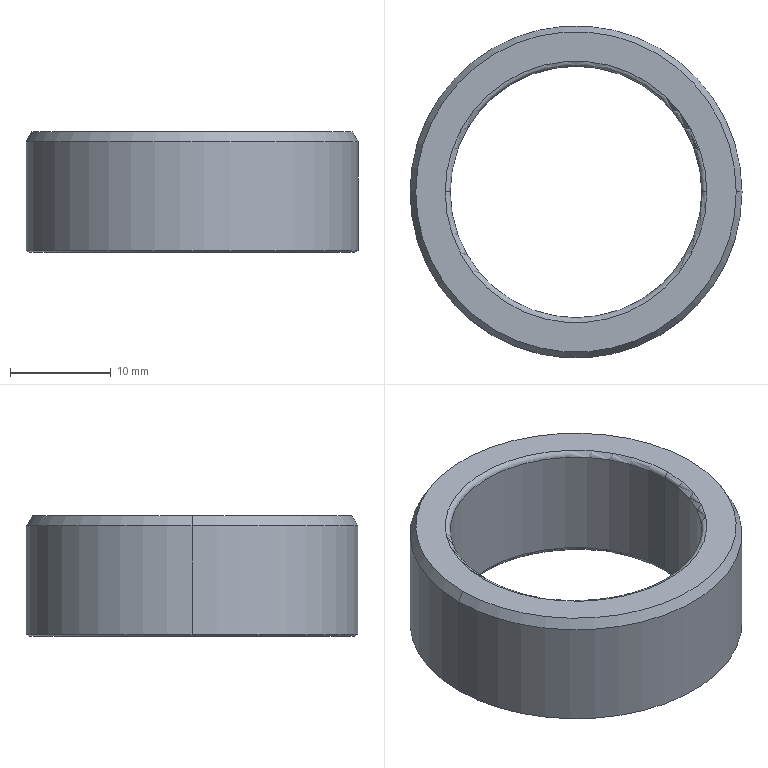Part | STEP file | Graphite bronze bushing JDB253312 | 1 solid | 14 faces | box 33 x 33 x 12 mm | volume 4332 mm3 | torus 4 | cone 4 | cylinder 4 | plane 2 | commonest cylinder face diameters 25 x2 33 x2
STEP:
#1=CARTESIAN_POINT('',(0.,0.,0.));
#2=DIRECTION('',(0.,0.,1.));
#3=DIRECTION('',(1.,0.,0.));
#4=AXIS2_PLACEMENT_3D('',#1,#2,#3);
#5=CARTESIAN_POINT('',(-12.5,0.,-5.5));
#6=VERTEX_POINT('',#5);
#7=CARTESIAN_POINT('',(12.5,0.,-5.5));
#8=VERTEX_POINT('',#7);
#9=CARTESIAN_POINT('',(0.,0.,-5.5));
#10=DIRECTION('',(0.,0.,-1.));
#11=DIRECTION('',(1.,0.,0.));
#12=AXIS2_PLACEMENT_3D('',#9,#10,#11);
#13=CIRCLE('',#12,12.5);
#14=CARTESIAN_POINT('',(0.,0.,-5.5));
#15=DIRECTION('',(0.,0.,1.));
#16=DIRECTION('',(1.,0.,0.));
#17=AXIS2_PLACEMENT_3D('',#14,#15,#16);
#18=TOROIDAL_SURFACE('',#17,13.,0.5);
#19=CARTESIAN_POINT('',(6.283,3.142));
#20=DIRECTION('',(-1.,0.));
#21=VECTOR('',#20,1.);
#22=LINE('',#19,#21);
#23=(GEOMETRIC_REPRESENTATION_CONTEXT(2)PARAMETRIC_REPRESENTATION_CONTEXT()REPRESENTATION_CONTEXT('',''));
#24=DEFINITIONAL_REPRESENTATION('',(#22),#23);
#25=PCURVE('',#18,#24);
#26=CARTESIAN_POINT('',(0.,0.,6.));
#27=DIRECTION('',(0.,0.,-1.));
#28=DIRECTION('',(-1.,0.,0.));
#29=AXIS2_PLACEMENT_3D('',#26,#27,#28);
#30=CYLINDRICAL_SURFACE('',#29,12.5);
#31=CARTESIAN_POINT('',(-3.142,11.5));
#32=DIRECTION('',(1.,0.));
#33=VECTOR('',#32,1.);
#34=LINE('',#31,#33);
#35=(GEOMETRIC_REPRESENTATION_CONTEXT(2)PARAMETRIC_REPRESENTATION_CONTEXT()REPRESENTATION_CONTEXT('',''));
#36=DEFINITIONAL_REPRESENTATION('',(#34),#35);
#37=PCURVE('',#30,#36);
#38=SURFACE_CURVE('',#13,(#25,#37),.PCURVE_S1.);
#39=EDGE_CURVE('',#6,#8,#38,.T.);
#40=ORIENTED_EDGE('',*,*,#39,.F.);
#41=CARTESIAN_POINT('',(-13.,0.,-6.));
#42=VERTEX_POINT('',#41);
#43=CARTESIAN_POINT('',(-13.,0.,-5.5));
#44=DIRECTION('',(0.,1.,0.));
#45=DIRECTION('',(-1.,0.,0.));
#46=AXIS2_PLACEMENT_3D('',#43,#44,#45);
#47=CIRCLE('',#46,0.5);
#48=CARTESIAN_POINT('',(3.142,0.));
#49=DIRECTION('',(0.,1.));
#50=VECTOR('',#49,1.);
#51=LINE('',#48,#50);
#52=(GEOMETRIC_REPRESENTATION_CONTEXT(2)PARAMETRIC_REPRESENTATION_CONTEXT()REPRESENTATION_CONTEXT('',''));
#53=DEFINITIONAL_REPRESENTATION('',(#51),#52);
#54=PCURVE('',#18,#53);
#55=CARTESIAN_POINT('',(0.,0.,-5.5));
#56=DIRECTION('',(0.,0.,1.));
#57=DIRECTION('',(1.,0.,0.));
#58=AXIS2_PLACEMENT_3D('',#55,#56,#57);
#59=TOROIDAL_SURFACE('',#58,13.,0.5);
#60=CARTESIAN_POINT('',(3.142,0.));
#61=DIRECTION('',(0.,1.));
#62=VECTOR('',#61,1.);
#63=LINE('',#60,#62);
#64=(GEOMETRIC_REPRESENTATION_CONTEXT(2)PARAMETRIC_REPRESENTATION_CONTEXT()REPRESENTATION_CONTEXT('',''));
#65=DEFINITIONAL_REPRESENTATION('',(#63),#64);
#66=PCURVE('',#59,#65);
#67=SURFACE_CURVE('',#47,(#54,#66),.PCURVE_S1.);
#68=EDGE_CURVE('',#6,#42,#67,.T.);
#69=ORIENTED_EDGE('',*,*,#68,.T.);
#70=CARTESIAN_POINT('',(13.,0.,-6.));
#71=VERTEX_POINT('',#70);
#72=CARTESIAN_POINT('',(0.,0.,-6.));
#73=DIRECTION('',(0.,0.,1.));
#74=DIRECTION('',(1.,0.,0.));
#75=AXIS2_PLACEMENT_3D('',#72,#73,#74);
#76=CIRCLE('',#75,13.);
#77=CARTESIAN_POINT('',(0.,4.712));
#78=DIRECTION('',(1.,0.));
#79=VECTOR('',#78,1.);
#80=LINE('',#77,#79);
#81=(GEOMETRIC_REPRESENTATION_CONTEXT(2)PARAMETRIC_REPRESENTATION_CONTEXT()REPRESENTATION_CONTEXT('',''));
#82=DEFINITIONAL_REPRESENTATION('',(#80),#81);
#83=PCURVE('',#18,#82);
#84=CARTESIAN_POINT('',(0.,0.,-6.));
#85=DIRECTION('',(0.,0.,1.));
#86=DIRECTION('',(1.,0.,0.));
#87=AXIS2_PLACEMENT_3D('',#84,#85,#86);
#88=PLANE('',#87);
#89=CARTESIAN_POINT('',(0.,0.));
#90=DIRECTION('',(1.,0.));
#91=AXIS2_PLACEMENT_2D('',#89,#90);
#92=CIRCLE('',#91,13.);
#93=(GEOMETRIC_REPRESENTATION_CONTEXT(2)PARAMETRIC_REPRESENTATION_CONTEXT()REPRESENTATION_CONTEXT('',''));
#94=DEFINITIONAL_REPRESENTATION('',(#92),#93);
#95=PCURVE('',#88,#94);
#96=SURFACE_CURVE('',#76,(#83,#95),.PCURVE_S1.);
#97=EDGE_CURVE('',#71,#42,#96,.T.);
#98=ORIENTED_EDGE('',*,*,#97,.F.);
#99=CARTESIAN_POINT('',(13.,0.,-5.5));
#100=DIRECTION('',(0.,-1.,0.));
#101=DIRECTION('',(0.,0.,-1.));
#102=AXIS2_PLACEMENT_3D('',#99,#100,#101);
#103=CIRCLE('',#102,0.5);
#104=CARTESIAN_POINT('',(0.,-1.571));
#105=DIRECTION('',(0.,1.));
#106=VECTOR('',#105,1.);
#107=LINE('',#104,#106);
#108=(GEOMETRIC_REPRESENTATION_CONTEXT(2)PARAMETRIC_REPRESENTATION_CONTEXT()REPRESENTATION_CONTEXT('',''));
#109=DEFINITIONAL_REPRESENTATION('',(#107),#108);
#110=PCURVE('',#18,#109);
#111=CARTESIAN_POINT('',(6.283,-1.571));
#112=DIRECTION('',(0.,1.));
#113=VECTOR('',#112,1.);
#114=LINE('',#111,#113);
#115=(GEOMETRIC_REPRESENTATION_CONTEXT(2)PARAMETRIC_REPRESENTATION_CONTEXT()REPRESENTATION_CONTEXT('',''));
#116=DEFINITIONAL_REPRESENTATION('',(#114),#115);
#117=PCURVE('',#59,#116);
#118=SURFACE_CURVE('',#103,(#110,#117),.PCURVE_S1.);
#119=EDGE_CURVE('',#8,#71,#118,.T.);
#120=ORIENTED_EDGE('',*,*,#119,.F.);
#121=EDGE_LOOP('',(#40,#69,#98,#120));
#122=FACE_BOUND('',#121,.T.);
#123=ADVANCED_FACE('',(#122),#18,.T.);
#124=CARTESIAN_POINT('',(-13.,0.,6.));
#125=VERTEX_POINT('',#124);
#126=CARTESIAN_POINT('',(13.,0.,6.));
#127=VERTEX_POINT('',#126);
#128=CARTESIAN_POINT('',(0.,0.,6.));
#129=DIRECTION('',(0.,0.,-1.));
#130=DIRECTION('',(1.,0.,0.));
#131=AXIS2_PLACEMENT_3D('',#128,#129,#130);
#132=CIRCLE('',#131,13.);
#133=CARTESIAN_POINT('',(0.,0.,5.5));
#134=DIRECTION('',(0.,0.,1.));
#135=DIRECTION('',(1.,0.,0.));
#136=AXIS2_PLACEMENT_3D('',#133,#134,#135);
#137=TOROIDAL_SURFACE('',#136,13.,0.5);
#138=CARTESIAN_POINT('',(6.283,1.571));
#139=DIRECTION('',(-1.,0.));
#140=VECTOR('',#139,1.);
#141=LINE('',#138,#140);
#142=(GEOMETRIC_REPRESENTATION_CONTEXT(2)PARAMETRIC_REPRESENTATION_CONTEXT()REPRESENTATION_CONTEXT('',''));
#143=DEFINITIONAL_REPRESENTATION('',(#141),#142);
#144=PCURVE('',#137,#143);
#145=CARTESIAN_POINT('',(0.,0.,6.));
#146=DIRECTION('',(0.,0.,1.));
#147=DIRECTION('',(1.,0.,0.));
#148=AXIS2_PLACEMENT_3D('',#145,#146,#147);
#149=PLANE('',#148);
#150=CARTESIAN_POINT('',(13.,0.));
#151=CARTESIAN_POINT('',(13.,-22.517));
#152=CARTESIAN_POINT('',(-6.5,-11.258));
#153=CARTESIAN_POINT('',(-26.,0.));
#154=CARTESIAN_POINT('',(-6.5,11.258));
#155=CARTESIAN_POINT('',(13.,22.517));
#156=CARTESIAN_POINT('',(13.,0.));
#157=(BOUNDED_CURVE()B_SPLINE_CURVE(2,(#150,#151,#152,#153,#154,#155,#156),.UNSPECIFIED.,.T.,.F.)B_SPLINE_CURVE_WITH_KNOTS((1,2,2,2,2,1),(-2.094,0.,2.094,4.189,6.283,8.378),.UNSPECIFIED.)CURVE()GEOMETRIC_REPRESENTATION_ITEM()RATIONAL_B_SPLINE_CURVE((1.,0.5,1.,0.5,1.,0.5,1.))REPRESENTATION_ITEM(''));
#158=(GEOMETRIC_REPRESENTATION_CONTEXT(2)PARAMETRIC_REPRESENTATION_CONTEXT()REPRESENTATION_CONTEXT('',''));
#159=DEFINITIONAL_REPRESENTATION('',(#157),#158);
#160=PCURVE('',#149,#159);
#161=SURFACE_CURVE('',#132,(#144,#160),.PCURVE_S1.);
#162=EDGE_CURVE('',#125,#127,#161,.T.);
#163=ORIENTED_EDGE('',*,*,#162,.F.);
#164=CARTESIAN_POINT('',(-12.5,0.,5.5));
#165=VERTEX_POINT('',#164);
#166=CARTESIAN_POINT('',(-13.,0.,5.5));
#167=DIRECTION('',(0.,1.,0.));
#168=DIRECTION('',(-1.,0.,0.));
#169=AXIS2_PLACEMENT_3D('',#166,#167,#168);
#170=CIRCLE('',#169,0.5);
#171=CARTESIAN_POINT('',(3.142,0.));
#172=DIRECTION('',(0.,1.));
#173=VECTOR('',#172,1.);
#174=LINE('',#171,#173);
#175=(GEOMETRIC_REPRESENTATION_CONTEXT(2)PARAMETRIC_REPRESENTATION_CONTEXT()REPRESENTATION_CONTEXT('',''));
#176=DEFINITIONAL_REPRESENTATION('',(#174),#175);
#177=PCURVE('',#137,#176);
#178=CARTESIAN_POINT('',(0.,0.,5.5));
#179=DIRECTION('',(0.,0.,1.));
#180=DIRECTION('',(1.,0.,0.));
#181=AXIS2_PLACEMENT_3D('',#178,#179,#180);
#182=TOROIDAL_SURFACE('',#181,13.,0.5);
#183=CARTESIAN_POINT('',(3.142,0.));
#184=DIRECTION('',(0.,1.));
#185=VECTOR('',#184,1.);
#186=LINE('',#183,#185);
#187=(GEOMETRIC_REPRESENTATION_CONTEXT(2)PARAMETRIC_REPRESENTATION_CONTEXT()REPRESENTATION_CONTEXT('',''));
#188=DEFINITIONAL_REPRESENTATION('',(#186),#187);
#189=PCURVE('',#182,#188);
#190=SURFACE_CURVE('',#170,(#177,#189),.PCURVE_S1.);
#191=EDGE_CURVE('',#125,#165,#190,.T.);
#192=ORIENTED_EDGE('',*,*,#191,.T.);
#193=CARTESIAN_POINT('',(12.5,0.,5.5));
#194=VERTEX_POINT('',#193);
#195=CARTESIAN_POINT('',(0.,0.,5.5));
#196=DIRECTION('',(0.,0.,1.));
#197=DIRECTION('',(1.,0.,0.));
#198=AXIS2_PLACEMENT_3D('',#195,#196,#197);
#199=CIRCLE('',#198,12.5);
#200=CARTESIAN_POINT('',(0.,3.142));
#201=DIRECTION('',(1.,0.));
#202=VECTOR('',#201,1.);
#203=LINE('',#200,#202);
#204=(GEOMETRIC_REPRESENTATION_CONTEXT(2)PARAMETRIC_REPRESENTATION_CONTEXT()REPRESENTATION_CONTEXT('',''));
#205=DEFINITIONAL_REPRESENTATION('',(#203),#204);
#206=PCURVE('',#137,#205);
#207=CARTESIAN_POINT('',(3.142,0.5));
#208=DIRECTION('',(-1.,0.));
#209=VECTOR('',#208,1.);
#210=LINE('',#207,#209);
#211=(GEOMETRIC_REPRESENTATION_CONTEXT(2)PARAMETRIC_REPRESENTATION_CONTEXT()REPRESENTATION_CONTEXT('',''));
#212=DEFINITIONAL_REPRESENTATION('',(#210),#211);
#213=PCURVE('',#30,#212);
#214=SURFACE_CURVE('',#199,(#206,#213),.PCURVE_S1.);
#215=EDGE_CURVE('',#194,#165,#214,.T.);
#216=ORIENTED_EDGE('',*,*,#215,.F.);
#217=CARTESIAN_POINT('',(13.,0.,5.5));
#218=DIRECTION('',(0.,-1.,0.));
#219=DIRECTION('',(0.,0.,-1.));
#220=AXIS2_PLACEMENT_3D('',#217,#218,#219);
#221=CIRCLE('',#220,0.5);
#222=CARTESIAN_POINT('',(0.,-1.571));
#223=DIRECTION('',(0.,1.));
#224=VECTOR('',#223,1.);
#225=LINE('',#222,#224);
#226=(GEOMETRIC_REPRESENTATION_CONTEXT(2)PARAMETRIC_REPRESENTATION_CONTEXT()REPRESENTATION_CONTEXT('',''));
#227=DEFINITIONAL_REPRESENTATION('',(#225),#226);
#228=PCURVE('',#137,#227);
#229=CARTESIAN_POINT('',(6.283,-1.571));
#230=DIRECTION('',(0.,1.));
#231=VECTOR('',#230,1.);
#232=LINE('',#229,#231);
#233=(GEOMETRIC_REPRESENTATION_CONTEXT(2)PARAMETRIC_REPRESENTATION_CONTEXT()REPRESENTATION_CONTEXT('',''));
#234=DEFINITIONAL_REPRESENTATION('',(#232),#233);
#235=PCURVE('',#182,#234);
#236=SURFACE_CURVE('',#221,(#228,#235),.PCURVE_S1.);
#237=EDGE_CURVE('',#127,#194,#236,.T.);
#238=ORIENTED_EDGE('',*,*,#237,.F.);
#239=EDGE_LOOP('',(#163,#192,#216,#238));
#240=FACE_BOUND('',#239,.T.);
#241=ADVANCED_FACE('',(#240),#137,.T.);
#242=CARTESIAN_POINT('',(-16.2,0.,-6.));
#243=VERTEX_POINT('',#242);
#244=CARTESIAN_POINT('',(16.2,0.,-6.));
#245=VERTEX_POINT('',#244);
#246=CARTESIAN_POINT('',(0.,0.,-6.));
#247=DIRECTION('',(0.,0.,-1.));
#248=DIRECTION('',(1.,0.,0.));
#249=AXIS2_PLACEMENT_3D('',#246,#247,#248);
#250=CIRCLE('',#249,16.2);
#251=CARTESIAN_POINT('',(0.,0.,-5.827));
#252=DIRECTION('',(0.,0.,1.));
#253=DIRECTION('',(1.,0.,0.));
#254=AXIS2_PLACEMENT_3D('',#251,#252,#253);
#255=CONICAL_SURFACE('',#254,16.5,1.047);
#256=CARTESIAN_POINT('',(6.283,-0.1732));
#257=DIRECTION('',(-1.,0.));
#258=VECTOR('',#257,1.);
#259=LINE('',#256,#258);
#260=(GEOMETRIC_REPRESENTATION_CONTEXT(2)PARAMETRIC_REPRESENTATION_CONTEXT()REPRESENTATION_CONTEXT('',''));
#261=DEFINITIONAL_REPRESENTATION('',(#259),#260);
#262=PCURVE('',#255,#261);
#263=CARTESIAN_POINT('',(16.2,0.));
#264=CARTESIAN_POINT('',(16.2,-28.059));
#265=CARTESIAN_POINT('',(-8.1,-14.03));
#266=CARTESIAN_POINT('',(-32.4,0.));
#267=CARTESIAN_POINT('',(-8.1,14.03));
#268=CARTESIAN_POINT('',(16.2,28.059));
#269=CARTESIAN_POINT('',(16.2,0.));
#270=(BOUNDED_CURVE()B_SPLINE_CURVE(2,(#263,#264,#265,#266,#267,#268,#269),.UNSPECIFIED.,.T.,.F.)B_SPLINE_CURVE_WITH_KNOTS((1,2,2,2,2,1),(-2.094,0.,2.094,4.189,6.283,8.378),.UNSPECIFIED.)CURVE()GEOMETRIC_REPRESENTATION_ITEM()RATIONAL_B_SPLINE_CURVE((1.,0.5,1.,0.5,1.,0.5,1.))REPRESENTATION_ITEM(''));
#271=(GEOMETRIC_REPRESENTATION_CONTEXT(2)PARAMETRIC_REPRESENTATION_CONTEXT()REPRESENTATION_CONTEXT('',''));
#272=DEFINITIONAL_REPRESENTATION('',(#270),#271);
#273=PCURVE('',#88,#272);
#274=SURFACE_CURVE('',#250,(#262,#273),.PCURVE_S1.);
#275=EDGE_CURVE('',#243,#245,#274,.T.);
#276=ORIENTED_EDGE('',*,*,#275,.F.);
#277=CARTESIAN_POINT('',(-16.5,0.,-5.827));
#278=VERTEX_POINT('',#277);
#279=CARTESIAN_POINT('',(-16.5,0.,-5.827));
#280=DIRECTION('',(-0.866,0.,0.5));
#281=VECTOR('',#280,1.);
#282=LINE('',#279,#281);
#283=CARTESIAN_POINT('',(3.142,0.));
#284=DIRECTION('',(0.,1.));
#285=VECTOR('',#284,1.);
#286=LINE('',#283,#285);
#287=(GEOMETRIC_REPRESENTATION_CONTEXT(2)PARAMETRIC_REPRESENTATION_CONTEXT()REPRESENTATION_CONTEXT('',''));
#288=DEFINITIONAL_REPRESENTATION('',(#286),#287);
#289=PCURVE('',#255,#288);
#290=CARTESIAN_POINT('',(0.,0.,-5.827));
#291=DIRECTION('',(0.,0.,1.));
#292=DIRECTION('',(1.,0.,0.));
#293=AXIS2_PLACEMENT_3D('',#290,#291,#292);
#294=CONICAL_SURFACE('',#293,16.5,1.047);
#295=CARTESIAN_POINT('',(3.142,0.));
#296=DIRECTION('',(0.,1.));
#297=VECTOR('',#296,1.);
#298=LINE('',#295,#297);
#299=(GEOMETRIC_REPRESENTATION_CONTEXT(2)PARAMETRIC_REPRESENTATION_CONTEXT()REPRESENTATION_CONTEXT('',''));
#300=DEFINITIONAL_REPRESENTATION('',(#298),#299);
#301=PCURVE('',#294,#300);
#302=SURFACE_CURVE('',#282,(#289,#301),.PCURVE_S1.);
#303=EDGE_CURVE('',#243,#278,#302,.T.);
#304=ORIENTED_EDGE('',*,*,#303,.T.);
#305=CARTESIAN_POINT('',(16.5,0.,-5.827));
#306=VERTEX_POINT('',#305);
#307=CARTESIAN_POINT('',(0.,0.,-5.827));
#308=DIRECTION('',(0.,0.,1.));
#309=DIRECTION('',(1.,0.,0.));
#310=AXIS2_PLACEMENT_3D('',#307,#308,#309);
#311=CIRCLE('',#310,16.5);
#312=CARTESIAN_POINT('',(0.,0.));
#313=DIRECTION('',(1.,0.));
#314=VECTOR('',#313,1.);
#315=LINE('',#312,#314);
#316=(GEOMETRIC_REPRESENTATION_CONTEXT(2)PARAMETRIC_REPRESENTATION_CONTEXT()REPRESENTATION_CONTEXT('',''));
#317=DEFINITIONAL_REPRESENTATION('',(#315),#316);
#318=PCURVE('',#255,#317);
#319=CARTESIAN_POINT('',(0.,0.,6.));
#320=DIRECTION('',(0.,0.,-1.));
#321=DIRECTION('',(-1.,0.,0.));
#322=AXIS2_PLACEMENT_3D('',#319,#320,#321);
#323=CYLINDRICAL_SURFACE('',#322,16.5);
#324=CARTESIAN_POINT('',(3.142,11.827));
#325=DIRECTION('',(-1.,0.));
#326=VECTOR('',#325,1.);
#327=LINE('',#324,#326);
#328=(GEOMETRIC_REPRESENTATION_CONTEXT(2)PARAMETRIC_REPRESENTATION_CONTEXT()REPRESENTATION_CONTEXT('',''));
#329=DEFINITIONAL_REPRESENTATION('',(#327),#328);
#330=PCURVE('',#323,#329);
#331=SURFACE_CURVE('',#311,(#318,#330),.PCURVE_S1.);
#332=EDGE_CURVE('',#306,#278,#331,.T.);
#333=ORIENTED_EDGE('',*,*,#332,.F.);
#334=CARTESIAN_POINT('',(16.5,0.,-5.827));
#335=DIRECTION('',(0.866,0.,0.5));
#336=VECTOR('',#335,1.);
#337=LINE('',#334,#336);
#338=CARTESIAN_POINT('',(0.,0.));
#339=DIRECTION('',(0.,1.));
#340=VECTOR('',#339,1.);
#341=LINE('',#338,#340);
#342=(GEOMETRIC_REPRESENTATION_CONTEXT(2)PARAMETRIC_REPRESENTATION_CONTEXT()REPRESENTATION_CONTEXT('',''));
#343=DEFINITIONAL_REPRESENTATION('',(#341),#342);
#344=PCURVE('',#255,#343);
#345=CARTESIAN_POINT('',(6.283,0.));
#346=DIRECTION('',(0.,1.));
#347=VECTOR('',#346,1.);
#348=LINE('',#345,#347);
#349=(GEOMETRIC_REPRESENTATION_CONTEXT(2)PARAMETRIC_REPRESENTATION_CONTEXT()REPRESENTATION_CONTEXT('',''));
#350=DEFINITIONAL_REPRESENTATION('',(#348),#349);
#351=PCURVE('',#294,#350);
#352=SURFACE_CURVE('',#337,(#344,#351),.PCURVE_S1.);
#353=EDGE_CURVE('',#245,#306,#352,.T.);
#354=ORIENTED_EDGE('',*,*,#353,.F.);
#355=EDGE_LOOP('',(#276,#304,#333,#354));
#356=FACE_BOUND('',#355,.T.);
#357=ADVANCED_FACE('',(#356),#255,.T.);
#358=CARTESIAN_POINT('',(15.923,0.,6.));
#359=VERTEX_POINT('',#358);
#360=CARTESIAN_POINT('',(-15.923,0.,6.));
#361=VERTEX_POINT('',#360);
#362=CARTESIAN_POINT('',(0.,0.,6.));
#363=DIRECTION('',(0.,0.,1.));
#364=DIRECTION('',(1.,0.,0.));
#365=AXIS2_PLACEMENT_3D('',#362,#363,#364);
#366=CIRCLE('',#365,15.923);
#367=CARTESIAN_POINT('',(0.,0.,6.));
#368=DIRECTION('',(0.,0.,-1.));
#369=DIRECTION('',(-1.,0.,0.));
#370=AXIS2_PLACEMENT_3D('',#367,#368,#369);
#371=CONICAL_SURFACE('',#370,15.923,0.5236);
#372=CARTESIAN_POINT('',(3.142,0.));
#373=DIRECTION('',(-1.,0.));
#374=VECTOR('',#373,1.);
#375=LINE('',#372,#374);
#376=(GEOMETRIC_REPRESENTATION_CONTEXT(2)PARAMETRIC_REPRESENTATION_CONTEXT()REPRESENTATION_CONTEXT('',''));
#377=DEFINITIONAL_REPRESENTATION('',(#375),#376);
#378=PCURVE('',#371,#377);
#379=CARTESIAN_POINT('',(0.,0.));
#380=DIRECTION('',(1.,0.));
#381=AXIS2_PLACEMENT_2D('',#379,#380);
#382=CIRCLE('',#381,15.923);
#383=(GEOMETRIC_REPRESENTATION_CONTEXT(2)PARAMETRIC_REPRESENTATION_CONTEXT()REPRESENTATION_CONTEXT('',''));
#384=DEFINITIONAL_REPRESENTATION('',(#382),#383);
#385=PCURVE('',#149,#384);
#386=SURFACE_CURVE('',#366,(#378,#385),.PCURVE_S1.);
#387=EDGE_CURVE('',#359,#361,#386,.T.);
#388=ORIENTED_EDGE('',*,*,#387,.F.);
#389=CARTESIAN_POINT('',(16.5,0.,5.));
#390=VERTEX_POINT('',#389);
#391=CARTESIAN_POINT('',(15.923,0.,6.));
#392=DIRECTION('',(0.5,0.,-0.866));
#393=VECTOR('',#392,1.);
#394=LINE('',#391,#393);
#395=CARTESIAN_POINT('',(3.142,0.));
#396=DIRECTION('',(0.,1.));
#397=VECTOR('',#396,1.);
#398=LINE('',#395,#397);
#399=(GEOMETRIC_REPRESENTATION_CONTEXT(2)PARAMETRIC_REPRESENTATION_CONTEXT()REPRESENTATION_CONTEXT('',''));
#400=DEFINITIONAL_REPRESENTATION('',(#398),#399);
#401=PCURVE('',#371,#400);
#402=CARTESIAN_POINT('',(0.,0.,6.));
#403=DIRECTION('',(0.,0.,-1.));
#404=DIRECTION('',(-1.,0.,0.));
#405=AXIS2_PLACEMENT_3D('',#402,#403,#404);
#406=CONICAL_SURFACE('',#405,15.923,0.5236);
#407=CARTESIAN_POINT('',(3.142,0.));
#408=DIRECTION('',(0.,1.));
#409=VECTOR('',#408,1.);
#410=LINE('',#407,#409);
#411=(GEOMETRIC_REPRESENTATION_CONTEXT(2)PARAMETRIC_REPRESENTATION_CONTEXT()REPRESENTATION_CONTEXT('',''));
#412=DEFINITIONAL_REPRESENTATION('',(#410),#411);
#413=PCURVE('',#406,#412);
#414=SURFACE_CURVE('',#394,(#401,#413),.PCURVE_S1.);
#415=EDGE_CURVE('',#359,#390,#414,.T.);
#416=ORIENTED_EDGE('',*,*,#415,.T.);
#417=CARTESIAN_POINT('',(-16.5,0.,5.));
#418=VERTEX_POINT('',#417);
#419=CARTESIAN_POINT('',(0.,0.,5.));
#420=DIRECTION('',(0.,0.,-1.));
#421=DIRECTION('',(1.,0.,0.));
#422=AXIS2_PLACEMENT_3D('',#419,#420,#421);
#423=CIRCLE('',#422,16.5);
#424=CARTESIAN_POINT('',(-3.142,1.));
#425=DIRECTION('',(1.,0.));
#426=VECTOR('',#425,1.);
#427=LINE('',#424,#426);
#428=(GEOMETRIC_REPRESENTATION_CONTEXT(2)PARAMETRIC_REPRESENTATION_CONTEXT()REPRESENTATION_CONTEXT('',''));
#429=DEFINITIONAL_REPRESENTATION('',(#427),#428);
#430=PCURVE('',#371,#429);
#431=CARTESIAN_POINT('',(-3.142,1.));
#432=DIRECTION('',(1.,0.));
#433=VECTOR('',#432,1.);
#434=LINE('',#431,#433);
#435=(GEOMETRIC_REPRESENTATION_CONTEXT(2)PARAMETRIC_REPRESENTATION_CONTEXT()REPRESENTATION_CONTEXT('',''));
#436=DEFINITIONAL_REPRESENTATION('',(#434),#435);
#437=PCURVE('',#323,#436);
#438=SURFACE_CURVE('',#423,(#430,#437),.PCURVE_S1.);
#439=EDGE_CURVE('',#418,#390,#438,.T.);
#440=ORIENTED_EDGE('',*,*,#439,.F.);
#441=CARTESIAN_POINT('',(-15.923,0.,6.));
#442=DIRECTION('',(-0.5,0.,-0.866));
#443=VECTOR('',#442,1.);
#444=LINE('',#441,#443);
#445=CARTESIAN_POINT('',(0.,0.));
#446=DIRECTION('',(0.,1.));
#447=VECTOR('',#446,1.);
#448=LINE('',#445,#447);
#449=(GEOMETRIC_REPRESENTATION_CONTEXT(2)PARAMETRIC_REPRESENTATION_CONTEXT()REPRESENTATION_CONTEXT('',''));
#450=DEFINITIONAL_REPRESENTATION('',(#448),#449);
#451=PCURVE('',#371,#450);
#452=CARTESIAN_POINT('',(6.283,0.));
#453=DIRECTION('',(0.,1.));
#454=VECTOR('',#453,1.);
#455=LINE('',#452,#454);
#456=(GEOMETRIC_REPRESENTATION_CONTEXT(2)PARAMETRIC_REPRESENTATION_CONTEXT()REPRESENTATION_CONTEXT('',''));
#457=DEFINITIONAL_REPRESENTATION('',(#455),#456);
#458=PCURVE('',#406,#457);
#459=SURFACE_CURVE('',#444,(#451,#458),.PCURVE_S1.);
#460=EDGE_CURVE('',#361,#418,#459,.T.);
#461=ORIENTED_EDGE('',*,*,#460,.F.);
#462=EDGE_LOOP('',(#388,#416,#440,#461));
#463=FACE_BOUND('',#462,.T.);
#464=ADVANCED_FACE('',(#463),#371,.T.);
#465=CARTESIAN_POINT('',(-12.5,0.,6.));
#466=DIRECTION('',(0.,0.,-1.));
#467=VECTOR('',#466,1.);
#468=LINE('',#465,#467);
#469=CARTESIAN_POINT('',(0.,0.,6.));
#470=DIRECTION('',(0.,0.,-1.));
#471=DIRECTION('',(-1.,0.,0.));
#472=AXIS2_PLACEMENT_3D('',#469,#470,#471);
#473=CYLINDRICAL_SURFACE('',#472,12.5);
#474=CARTESIAN_POINT('',(6.283,0.));
#475=DIRECTION('',(0.,1.));
#476=VECTOR('',#475,1.);
#477=LINE('',#474,#476);
#478=(GEOMETRIC_REPRESENTATION_CONTEXT(2)PARAMETRIC_REPRESENTATION_CONTEXT()REPRESENTATION_CONTEXT('',''));
#479=DEFINITIONAL_REPRESENTATION('',(#477),#478);
#480=PCURVE('',#473,#479);
#481=CARTESIAN_POINT('',(0.,0.));
#482=DIRECTION('',(0.,1.));
#483=VECTOR('',#482,1.);
#484=LINE('',#481,#483);
#485=(GEOMETRIC_REPRESENTATION_CONTEXT(2)PARAMETRIC_REPRESENTATION_CONTEXT()REPRESENTATION_CONTEXT('',''));
#486=DEFINITIONAL_REPRESENTATION('',(#484),#485);
#487=PCURVE('',#30,#486);
#488=SURFACE_CURVE('',#468,(#480,#487),.PCURVE_S1.);
#489=EDGE_CURVE('',#165,#6,#488,.T.);
#490=ORIENTED_EDGE('',*,*,#489,.T.);
#491=CARTESIAN_POINT('',(0.,0.,-5.5));
#492=DIRECTION('',(0.,0.,-1.));
#493=DIRECTION('',(1.,0.,0.));
#494=AXIS2_PLACEMENT_3D('',#491,#492,#493);
#495=CIRCLE('',#494,12.5);
#496=CARTESIAN_POINT('',(3.142,11.5));
#497=DIRECTION('',(1.,0.));
#498=VECTOR('',#497,1.);
#499=LINE('',#496,#498);
#500=(GEOMETRIC_REPRESENTATION_CONTEXT(2)PARAMETRIC_REPRESENTATION_CONTEXT()REPRESENTATION_CONTEXT('',''));
#501=DEFINITIONAL_REPRESENTATION('',(#499),#500);
#502=PCURVE('',#473,#501);
#503=CARTESIAN_POINT('',(6.283,3.142));
#504=DIRECTION('',(-1.,0.));
#505=VECTOR('',#504,1.);
#506=LINE('',#503,#505);
#507=(GEOMETRIC_REPRESENTATION_CONTEXT(2)PARAMETRIC_REPRESENTATION_CONTEXT()REPRESENTATION_CONTEXT('',''));
#508=DEFINITIONAL_REPRESENTATION('',(#506),#507);
#509=PCURVE('',#59,#508);
#510=SURFACE_CURVE('',#495,(#502,#509),.PCURVE_S1.);
#511=EDGE_CURVE('',#8,#6,#510,.T.);
#512=ORIENTED_EDGE('',*,*,#511,.F.);
#513=CARTESIAN_POINT('',(12.5,0.,6.));
#514=DIRECTION('',(0.,0.,-1.));
#515=VECTOR('',#514,1.);
#516=LINE('',#513,#515);
#517=CARTESIAN_POINT('',(3.142,0.));
#518=DIRECTION('',(0.,1.));
#519=VECTOR('',#518,1.);
#520=LINE('',#517,#519);
#521=(GEOMETRIC_REPRESENTATION_CONTEXT(2)PARAMETRIC_REPRESENTATION_CONTEXT()REPRESENTATION_CONTEXT('',''));
#522=DEFINITIONAL_REPRESENTATION('',(#520),#521);
#523=PCURVE('',#473,#522);
#524=CARTESIAN_POINT('',(3.142,0.));
#525=DIRECTION('',(0.,1.));
#526=VECTOR('',#525,1.);
#527=LINE('',#524,#526);
#528=(GEOMETRIC_REPRESENTATION_CONTEXT(2)PARAMETRIC_REPRESENTATION_CONTEXT()REPRESENTATION_CONTEXT('',''));
#529=DEFINITIONAL_REPRESENTATION('',(#527),#528);
#530=PCURVE('',#30,#529);
#531=SURFACE_CURVE('',#516,(#523,#530),.PCURVE_S1.);
#532=EDGE_CURVE('',#194,#8,#531,.T.);
#533=ORIENTED_EDGE('',*,*,#532,.F.);
#534=CARTESIAN_POINT('',(0.,0.,5.5));
#535=DIRECTION('',(0.,0.,1.));
#536=DIRECTION('',(1.,0.,0.));
#537=AXIS2_PLACEMENT_3D('',#534,#535,#536);
#538=CIRCLE('',#537,12.5);
#539=CARTESIAN_POINT('',(9.425,0.5));
#540=DIRECTION('',(-1.,0.));
#541=VECTOR('',#540,1.);
#542=LINE('',#539,#541);
#543=(GEOMETRIC_REPRESENTATION_CONTEXT(2)PARAMETRIC_REPRESENTATION_CONTEXT()REPRESENTATION_CONTEXT('',''));
#544=DEFINITIONAL_REPRESENTATION('',(#542),#543);
#545=PCURVE('',#473,#544);
#546=CARTESIAN_POINT('',(0.,3.142));
#547=DIRECTION('',(1.,0.));
#548=VECTOR('',#547,1.);
#549=LINE('',#546,#548);
#550=(GEOMETRIC_REPRESENTATION_CONTEXT(2)PARAMETRIC_REPRESENTATION_CONTEXT()REPRESENTATION_CONTEXT('',''));
#551=DEFINITIONAL_REPRESENTATION('',(#549),#550);
#552=PCURVE('',#182,#551);
#553=SURFACE_CURVE('',#538,(#545,#552),.PCURVE_S1.);
#554=EDGE_CURVE('',#165,#194,#553,.T.);
#555=ORIENTED_EDGE('',*,*,#554,.F.);
#556=EDGE_LOOP('',(#490,#512,#533,#555));
#557=FACE_BOUND('',#556,.F.);
#558=ADVANCED_FACE('',(#557),#473,.F.);
#559=ORIENTED_EDGE('',*,*,#439,.T.);
#560=CARTESIAN_POINT('',(16.5,0.,6.));
#561=DIRECTION('',(0.,0.,-1.));
#562=VECTOR('',#561,1.);
#563=LINE('',#560,#562);
#564=CARTESIAN_POINT('',(3.142,0.));
#565=DIRECTION('',(0.,1.));
#566=VECTOR('',#565,1.);
#567=LINE('',#564,#566);
#568=(GEOMETRIC_REPRESENTATION_CONTEXT(2)PARAMETRIC_REPRESENTATION_CONTEXT()REPRESENTATION_CONTEXT('',''));
#569=DEFINITIONAL_REPRESENTATION('',(#567),#568);
#570=PCURVE('',#323,#569);
#571=CARTESIAN_POINT('',(0.,0.,6.));
#572=DIRECTION('',(0.,0.,-1.));
#573=DIRECTION('',(-1.,0.,0.));
#574=AXIS2_PLACEMENT_3D('',#571,#572,#573);
#575=CYLINDRICAL_SURFACE('',#574,16.5);
#576=CARTESIAN_POINT('',(3.142,0.));
#577=DIRECTION('',(0.,1.));
#578=VECTOR('',#577,1.);
#579=LINE('',#576,#578);
#580=(GEOMETRIC_REPRESENTATION_CONTEXT(2)PARAMETRIC_REPRESENTATION_CONTEXT()REPRESENTATION_CONTEXT('',''));
#581=DEFINITIONAL_REPRESENTATION('',(#579),#580);
#582=PCURVE('',#575,#581);
#583=SURFACE_CURVE('',#563,(#570,#582),.PCURVE_S1.);
#584=EDGE_CURVE('',#390,#306,#583,.T.);
#585=ORIENTED_EDGE('',*,*,#584,.T.);
#586=ORIENTED_EDGE('',*,*,#332,.T.);
#587=CARTESIAN_POINT('',(-16.5,0.,6.));
#588=DIRECTION('',(0.,0.,-1.));
#589=VECTOR('',#588,1.);
#590=LINE('',#587,#589);
#591=CARTESIAN_POINT('',(0.,0.));
#592=DIRECTION('',(0.,1.));
#593=VECTOR('',#592,1.);
#594=LINE('',#591,#593);
#595=(GEOMETRIC_REPRESENTATION_CONTEXT(2)PARAMETRIC_REPRESENTATION_CONTEXT()REPRESENTATION_CONTEXT('',''));
#596=DEFINITIONAL_REPRESENTATION('',(#594),#595);
#597=PCURVE('',#323,#596);
#598=CARTESIAN_POINT('',(6.283,0.));
#599=DIRECTION('',(0.,1.));
#600=VECTOR('',#599,1.);
#601=LINE('',#598,#600);
#602=(GEOMETRIC_REPRESENTATION_CONTEXT(2)PARAMETRIC_REPRESENTATION_CONTEXT()REPRESENTATION_CONTEXT('',''));
#603=DEFINITIONAL_REPRESENTATION('',(#601),#602);
#604=PCURVE('',#575,#603);
#605=SURFACE_CURVE('',#590,(#597,#604),.PCURVE_S1.);
#606=EDGE_CURVE('',#418,#278,#605,.T.);
#607=ORIENTED_EDGE('',*,*,#606,.F.);
#608=EDGE_LOOP('',(#559,#585,#586,#607));
#609=FACE_BOUND('',#608,.T.);
#610=ADVANCED_FACE('',(#609),#323,.T.);
#611=CARTESIAN_POINT('',(0.,0.,6.));
#612=DIRECTION('',(0.,0.,-1.));
#613=DIRECTION('',(1.,0.,0.));
#614=AXIS2_PLACEMENT_3D('',#611,#612,#613);
#615=CIRCLE('',#614,13.);
#616=CARTESIAN_POINT('',(13.,0.));
#617=CARTESIAN_POINT('',(13.,-22.517));
#618=CARTESIAN_POINT('',(-6.5,-11.258));
#619=CARTESIAN_POINT('',(-26.,0.));
#620=CARTESIAN_POINT('',(-6.5,11.258));
#621=CARTESIAN_POINT('',(13.,22.517));
#622=CARTESIAN_POINT('',(13.,0.));
#623=(BOUNDED_CURVE()B_SPLINE_CURVE(2,(#616,#617,#618,#619,#620,#621,#622),.UNSPECIFIED.,.T.,.F.)B_SPLINE_CURVE_WITH_KNOTS((1,2,2,2,2,1),(-2.094,0.,2.094,4.189,6.283,8.378),.UNSPECIFIED.)CURVE()GEOMETRIC_REPRESENTATION_ITEM()RATIONAL_B_SPLINE_CURVE((1.,0.5,1.,0.5,1.,0.5,1.))REPRESENTATION_ITEM(''));
#624=(GEOMETRIC_REPRESENTATION_CONTEXT(2)PARAMETRIC_REPRESENTATION_CONTEXT()REPRESENTATION_CONTEXT('',''));
#625=DEFINITIONAL_REPRESENTATION('',(#623),#624);
#626=PCURVE('',#149,#625);
#627=CARTESIAN_POINT('',(6.283,1.571));
#628=DIRECTION('',(-1.,0.));
#629=VECTOR('',#628,1.);
#630=LINE('',#627,#629);
#631=(GEOMETRIC_REPRESENTATION_CONTEXT(2)PARAMETRIC_REPRESENTATION_CONTEXT()REPRESENTATION_CONTEXT('',''));
#632=DEFINITIONAL_REPRESENTATION('',(#630),#631);
#633=PCURVE('',#182,#632);
#634=SURFACE_CURVE('',#615,(#626,#633),.PCURVE_S1.);
#635=EDGE_CURVE('',#127,#125,#634,.T.);
#636=ORIENTED_EDGE('',*,*,#635,.T.);
#637=ORIENTED_EDGE('',*,*,#162,.T.);
#638=EDGE_LOOP('',(#636,#637));
#639=FACE_BOUND('',#638,.T.);
#640=CARTESIAN_POINT('',(0.,0.,6.));
#641=DIRECTION('',(0.,0.,1.));
#642=DIRECTION('',(1.,0.,0.));
#643=AXIS2_PLACEMENT_3D('',#640,#641,#642);
#644=CIRCLE('',#643,15.923);
#645=CARTESIAN_POINT('',(0.,0.));
#646=DIRECTION('',(1.,0.));
#647=AXIS2_PLACEMENT_2D('',#645,#646);
#648=CIRCLE('',#647,15.923);
#649=(GEOMETRIC_REPRESENTATION_CONTEXT(2)PARAMETRIC_REPRESENTATION_CONTEXT()REPRESENTATION_CONTEXT('',''));
#650=DEFINITIONAL_REPRESENTATION('',(#648),#649);
#651=PCURVE('',#149,#650);
#652=CARTESIAN_POINT('',(9.425,0.));
#653=DIRECTION('',(-1.,0.));
#654=VECTOR('',#653,1.);
#655=LINE('',#652,#654);
#656=(GEOMETRIC_REPRESENTATION_CONTEXT(2)PARAMETRIC_REPRESENTATION_CONTEXT()REPRESENTATION_CONTEXT('',''));
#657=DEFINITIONAL_REPRESENTATION('',(#655),#656);
#658=PCURVE('',#406,#657);
#659=SURFACE_CURVE('',#644,(#651,#658),.PCURVE_S1.);
#660=EDGE_CURVE('',#361,#359,#659,.T.);
#661=ORIENTED_EDGE('',*,*,#660,.T.);
#662=ORIENTED_EDGE('',*,*,#387,.T.);
#663=EDGE_LOOP('',(#661,#662));
#664=FACE_BOUND('',#663,.T.);
#665=ADVANCED_FACE('',(#639,#664),#149,.T.);
#666=ORIENTED_EDGE('',*,*,#97,.T.);
#667=CARTESIAN_POINT('',(0.,0.,-6.));
#668=DIRECTION('',(0.,0.,1.));
#669=DIRECTION('',(1.,0.,0.));
#670=AXIS2_PLACEMENT_3D('',#667,#668,#669);
#671=CIRCLE('',#670,13.);
#672=CARTESIAN_POINT('',(0.,0.));
#673=DIRECTION('',(1.,0.));
#674=AXIS2_PLACEMENT_2D('',#672,#673);
#675=CIRCLE('',#674,13.);
#676=(GEOMETRIC_REPRESENTATION_CONTEXT(2)PARAMETRIC_REPRESENTATION_CONTEXT()REPRESENTATION_CONTEXT('',''));
#677=DEFINITIONAL_REPRESENTATION('',(#675),#676);
#678=PCURVE('',#88,#677);
#679=CARTESIAN_POINT('',(0.,4.712));
#680=DIRECTION('',(1.,0.));
#681=VECTOR('',#680,1.);
#682=LINE('',#679,#681);
#683=(GEOMETRIC_REPRESENTATION_CONTEXT(2)PARAMETRIC_REPRESENTATION_CONTEXT()REPRESENTATION_CONTEXT('',''));
#684=DEFINITIONAL_REPRESENTATION('',(#682),#683);
#685=PCURVE('',#59,#684);
#686=SURFACE_CURVE('',#671,(#678,#685),.PCURVE_S1.);
#687=EDGE_CURVE('',#42,#71,#686,.T.);
#688=ORIENTED_EDGE('',*,*,#687,.T.);
#689=EDGE_LOOP('',(#666,#688));
#690=FACE_BOUND('',#689,.T.);
#691=CARTESIAN_POINT('',(0.,0.,-6.));
#692=DIRECTION('',(0.,0.,-1.));
#693=DIRECTION('',(1.,0.,0.));
#694=AXIS2_PLACEMENT_3D('',#691,#692,#693);
#695=CIRCLE('',#694,16.2);
#696=CARTESIAN_POINT('',(16.2,0.));
#697=CARTESIAN_POINT('',(16.2,-28.059));
#698=CARTESIAN_POINT('',(-8.1,-14.03));
#699=CARTESIAN_POINT('',(-32.4,0.));
#700=CARTESIAN_POINT('',(-8.1,14.03));
#701=CARTESIAN_POINT('',(16.2,28.059));
#702=CARTESIAN_POINT('',(16.2,0.));
#703=(BOUNDED_CURVE()B_SPLINE_CURVE(2,(#696,#697,#698,#699,#700,#701,#702),.UNSPECIFIED.,.T.,.F.)B_SPLINE_CURVE_WITH_KNOTS((1,2,2,2,2,1),(-2.094,0.,2.094,4.189,6.283,8.378),.UNSPECIFIED.)CURVE()GEOMETRIC_REPRESENTATION_ITEM()RATIONAL_B_SPLINE_CURVE((1.,0.5,1.,0.5,1.,0.5,1.))REPRESENTATION_ITEM(''));
#704=(GEOMETRIC_REPRESENTATION_CONTEXT(2)PARAMETRIC_REPRESENTATION_CONTEXT()REPRESENTATION_CONTEXT('',''));
#705=DEFINITIONAL_REPRESENTATION('',(#703),#704);
#706=PCURVE('',#88,#705);
#707=CARTESIAN_POINT('',(6.283,-0.1732));
#708=DIRECTION('',(-1.,0.));
#709=VECTOR('',#708,1.);
#710=LINE('',#707,#709);
#711=(GEOMETRIC_REPRESENTATION_CONTEXT(2)PARAMETRIC_REPRESENTATION_CONTEXT()REPRESENTATION_CONTEXT('',''));
#712=DEFINITIONAL_REPRESENTATION('',(#710),#711);
#713=PCURVE('',#294,#712);
#714=SURFACE_CURVE('',#695,(#706,#713),.PCURVE_S1.);
#715=EDGE_CURVE('',#245,#243,#714,.T.);
#716=ORIENTED_EDGE('',*,*,#715,.T.);
#717=ORIENTED_EDGE('',*,*,#275,.T.);
#718=EDGE_LOOP('',(#716,#717));
#719=FACE_BOUND('',#718,.T.);
#720=ADVANCED_FACE('',(#690,#719),#88,.F.);
#721=ORIENTED_EDGE('',*,*,#584,.F.);
#722=CARTESIAN_POINT('',(0.,0.,5.));
#723=DIRECTION('',(0.,0.,-1.));
#724=DIRECTION('',(1.,0.,0.));
#725=AXIS2_PLACEMENT_3D('',#722,#723,#724);
#726=CIRCLE('',#725,16.5);
#727=CARTESIAN_POINT('',(3.142,1.));
#728=DIRECTION('',(1.,0.));
#729=VECTOR('',#728,1.);
#730=LINE('',#727,#729);
#731=(GEOMETRIC_REPRESENTATION_CONTEXT(2)PARAMETRIC_REPRESENTATION_CONTEXT()REPRESENTATION_CONTEXT('',''));
#732=DEFINITIONAL_REPRESENTATION('',(#730),#731);
#733=PCURVE('',#575,#732);
#734=CARTESIAN_POINT('',(3.142,1.));
#735=DIRECTION('',(1.,0.));
#736=VECTOR('',#735,1.);
#737=LINE('',#734,#736);
#738=(GEOMETRIC_REPRESENTATION_CONTEXT(2)PARAMETRIC_REPRESENTATION_CONTEXT()REPRESENTATION_CONTEXT('',''));
#739=DEFINITIONAL_REPRESENTATION('',(#737),#738);
#740=PCURVE('',#406,#739);
#741=SURFACE_CURVE('',#726,(#733,#740),.PCURVE_S1.);
#742=EDGE_CURVE('',#390,#418,#741,.T.);
#743=ORIENTED_EDGE('',*,*,#742,.T.);
#744=ORIENTED_EDGE('',*,*,#606,.T.);
#745=CARTESIAN_POINT('',(0.,0.,-5.827));
#746=DIRECTION('',(0.,0.,1.));
#747=DIRECTION('',(1.,0.,0.));
#748=AXIS2_PLACEMENT_3D('',#745,#746,#747);
#749=CIRCLE('',#748,16.5);
#750=CARTESIAN_POINT('',(9.425,11.827));
#751=DIRECTION('',(-1.,0.));
#752=VECTOR('',#751,1.);
#753=LINE('',#750,#752);
#754=(GEOMETRIC_REPRESENTATION_CONTEXT(2)PARAMETRIC_REPRESENTATION_CONTEXT()REPRESENTATION_CONTEXT('',''));
#755=DEFINITIONAL_REPRESENTATION('',(#753),#754);
#756=PCURVE('',#575,#755);
#757=CARTESIAN_POINT('',(0.,0.));
#758=DIRECTION('',(1.,0.));
#759=VECTOR('',#758,1.);
#760=LINE('',#757,#759);
#761=(GEOMETRIC_REPRESENTATION_CONTEXT(2)PARAMETRIC_REPRESENTATION_CONTEXT()REPRESENTATION_CONTEXT('',''));
#762=DEFINITIONAL_REPRESENTATION('',(#760),#761);
#763=PCURVE('',#294,#762);
#764=SURFACE_CURVE('',#749,(#756,#763),.PCURVE_S1.);
#765=EDGE_CURVE('',#278,#306,#764,.T.);
#766=ORIENTED_EDGE('',*,*,#765,.T.);
#767=EDGE_LOOP('',(#721,#743,#744,#766));
#768=FACE_BOUND('',#767,.T.);
#769=ADVANCED_FACE('',(#768),#575,.T.);
#770=ORIENTED_EDGE('',*,*,#39,.F.);
#771=ORIENTED_EDGE('',*,*,#489,.F.);
#772=ORIENTED_EDGE('',*,*,#215,.F.);
#773=ORIENTED_EDGE('',*,*,#532,.T.);
#774=EDGE_LOOP('',(#770,#771,#772,#773));
#775=FACE_BOUND('',#774,.F.);
#776=ADVANCED_FACE('',(#775),#30,.F.);
#777=ORIENTED_EDGE('',*,*,#415,.F.);
#778=ORIENTED_EDGE('',*,*,#660,.F.);
#779=ORIENTED_EDGE('',*,*,#460,.T.);
#780=ORIENTED_EDGE('',*,*,#742,.F.);
#781=EDGE_LOOP('',(#777,#778,#779,#780));
#782=FACE_BOUND('',#781,.T.);
#783=ADVANCED_FACE('',(#782),#406,.T.);
#784=ORIENTED_EDGE('',*,*,#303,.F.);
#785=ORIENTED_EDGE('',*,*,#715,.F.);
#786=ORIENTED_EDGE('',*,*,#353,.T.);
#787=ORIENTED_EDGE('',*,*,#765,.F.);
#788=EDGE_LOOP('',(#784,#785,#786,#787));
#789=FACE_BOUND('',#788,.T.);
#790=ADVANCED_FACE('',(#789),#294,.T.);
#791=ORIENTED_EDGE('',*,*,#191,.F.);
#792=ORIENTED_EDGE('',*,*,#635,.F.);
#793=ORIENTED_EDGE('',*,*,#237,.T.);
#794=ORIENTED_EDGE('',*,*,#554,.F.);
#795=EDGE_LOOP('',(#791,#792,#793,#794));
#796=FACE_BOUND('',#795,.T.);
#797=ADVANCED_FACE('',(#796),#182,.T.);
#798=ORIENTED_EDGE('',*,*,#68,.F.);
#799=ORIENTED_EDGE('',*,*,#511,.F.);
#800=ORIENTED_EDGE('',*,*,#119,.T.);
#801=ORIENTED_EDGE('',*,*,#687,.F.);
#802=EDGE_LOOP('',(#798,#799,#800,#801));
#803=FACE_BOUND('',#802,.T.);
#804=ADVANCED_FACE('',(#803),#59,.T.);
#805=CLOSED_SHELL('',(#123,#241,#357,#464,#558,#610,#665,#720,#769,#776,#783,#790,#797,#804));
#806=MANIFOLD_SOLID_BREP('',#805);
#807=(LENGTH_UNIT()NAMED_UNIT(*)SI_UNIT(.MILLI.,.METRE.));
#808=UNCERTAINTY_MEASURE_WITH_UNIT(LENGTH_MEASURE(0.0000001),#807,'','');
#809=(NAMED_UNIT(*)PLANE_ANGLE_UNIT()SI_UNIT($,.RADIAN.));
#810=(NAMED_UNIT(*)SI_UNIT($,.STERADIAN.)SOLID_ANGLE_UNIT());
#811=(GEOMETRIC_REPRESENTATION_CONTEXT(3)GLOBAL_UNCERTAINTY_ASSIGNED_CONTEXT((#808))GLOBAL_UNIT_ASSIGNED_CONTEXT((#807,#809,#810))REPRESENTATION_CONTEXT('',''));
#812=ADVANCED_BREP_SHAPE_REPRESENTATION('',(#4,#806),#811);